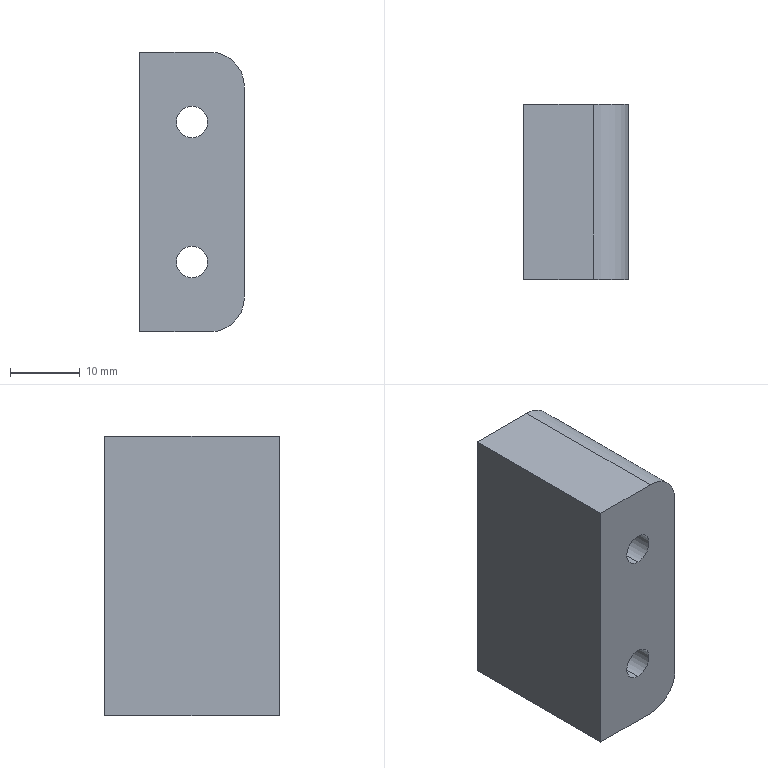Part | SolidWorks | features Extrusion 1, Fillet 1, HoleWzd 1 | 1 solid | 22 faces | box 15 x 25 x 40 mm | volume 13620 mm3 | cylinder 10 | plane 8 | cone 4 | commonest cylinder face diameters 4.5 x4 8 x4 10 x2
STEP:
#1=CARTESIAN_POINT('',(0.,24.975,-14.));
#2=VERTEX_POINT('',#1);
#3=CARTESIAN_POINT('',(0.,24.975,-6.));
#4=VERTEX_POINT('',#3);
#5=CARTESIAN_POINT('',(0.,24.975,-10.));
#6=DIRECTION('',(0.,1.,0.));
#7=DIRECTION('',(0.,0.,1.));
#8=AXIS2_PLACEMENT_3D('',#5,#6,#7);
#9=CIRCLE('',#8,4.);
#10=EDGE_CURVE('',#2,#4,#9,.T.);
#11=ORIENTED_EDGE('',*,*,#10,.F.);
#12=CARTESIAN_POINT('',(0.,25.,-14.025));
#13=VERTEX_POINT('',#12);
#14=CARTESIAN_POINT('',(0.,25.,-14.025));
#15=DIRECTION('',(0.,0.7071,-0.7071));
#16=VECTOR('',#15,1000.);
#17=LINE('',#14,#16);
#18=EDGE_CURVE('',#2,#13,#17,.T.);
#19=ORIENTED_EDGE('',*,*,#18,.T.);
#20=CARTESIAN_POINT('',(0.,25.,-5.975));
#21=VERTEX_POINT('',#20);
#22=CARTESIAN_POINT('',(0.,25.,-10.));
#23=DIRECTION('',(0.,1.,0.));
#24=DIRECTION('',(0.,0.,1.));
#25=AXIS2_PLACEMENT_3D('',#22,#23,#24);
#26=CIRCLE('',#25,4.025);
#27=EDGE_CURVE('',#13,#21,#26,.T.);
#28=ORIENTED_EDGE('',*,*,#27,.T.);
#29=CARTESIAN_POINT('',(0.,25.,-5.975));
#30=DIRECTION('',(0.,0.7071,0.7071));
#31=VECTOR('',#30,1000.);
#32=LINE('',#29,#31);
#33=EDGE_CURVE('',#4,#21,#32,.T.);
#34=ORIENTED_EDGE('',*,*,#33,.F.);
#35=EDGE_LOOP('',(#11,#19,#28,#34));
#36=FACE_OUTER_BOUND('',#35,.T.);
#37=CARTESIAN_POINT('',(0.,25.,-10.));
#38=DIRECTION('',(0.,1.,0.));
#39=DIRECTION('',(0.,0.,1.));
#40=AXIS2_PLACEMENT_3D('',#37,#38,#39);
#41=CONICAL_SURFACE('',#40,4.025,0.7854);
#42=ADVANCED_FACE('',(#36),#41,.F.);
#43=CARTESIAN_POINT('',(0.,20.4,-14.));
#44=VERTEX_POINT('',#43);
#45=CARTESIAN_POINT('',(0.,20.4,-6.));
#46=VERTEX_POINT('',#45);
#47=CARTESIAN_POINT('',(0.,20.4,-10.));
#48=DIRECTION('',(0.,1.,0.));
#49=DIRECTION('',(0.,0.,1.));
#50=AXIS2_PLACEMENT_3D('',#47,#48,#49);
#51=CIRCLE('',#50,4.);
#52=EDGE_CURVE('',#44,#46,#51,.T.);
#53=ORIENTED_EDGE('',*,*,#52,.F.);
#54=CARTESIAN_POINT('',(0.,25.,-14.));
#55=DIRECTION('',(0.,1.,0.));
#56=VECTOR('',#55,1000.);
#57=LINE('',#54,#56);
#58=EDGE_CURVE('',#44,#2,#57,.T.);
#59=ORIENTED_EDGE('',*,*,#58,.T.);
#60=ORIENTED_EDGE('',*,*,#10,.T.);
#61=CARTESIAN_POINT('',(0.,25.,-6.));
#62=DIRECTION('',(0.,1.,0.));
#63=VECTOR('',#62,1000.);
#64=LINE('',#61,#63);
#65=EDGE_CURVE('',#46,#4,#64,.T.);
#66=ORIENTED_EDGE('',*,*,#65,.F.);
#67=EDGE_LOOP('',(#53,#59,#60,#66));
#68=FACE_OUTER_BOUND('',#67,.T.);
#69=CARTESIAN_POINT('',(0.,25.,-10.));
#70=DIRECTION('',(0.,1.,0.));
#71=DIRECTION('',(0.,0.,1.));
#72=AXIS2_PLACEMENT_3D('',#69,#70,#71);
#73=CYLINDRICAL_SURFACE('',#72,4.);
#74=ADVANCED_FACE('',(#68),#73,.F.);
#75=CARTESIAN_POINT('',(0.,0.,-12.25));
#76=VERTEX_POINT('',#75);
#77=CARTESIAN_POINT('',(0.,0.,-7.75));
#78=VERTEX_POINT('',#77);
#79=CARTESIAN_POINT('',(0.,0.,-10.));
#80=DIRECTION('',(0.,1.,0.));
#81=DIRECTION('',(0.,0.,1.));
#82=AXIS2_PLACEMENT_3D('',#79,#80,#81);
#83=CIRCLE('',#82,2.25);
#84=EDGE_CURVE('',#76,#78,#83,.T.);
#85=ORIENTED_EDGE('',*,*,#84,.F.);
#86=CARTESIAN_POINT('',(0.,20.4,-12.25));
#87=VERTEX_POINT('',#86);
#88=CARTESIAN_POINT('',(0.,25.,-12.25));
#89=DIRECTION('',(0.,1.,0.));
#90=VECTOR('',#89,1000.);
#91=LINE('',#88,#90);
#92=EDGE_CURVE('',#76,#87,#91,.T.);
#93=ORIENTED_EDGE('',*,*,#92,.T.);
#94=CARTESIAN_POINT('',(0.,20.4,-7.75));
#95=VERTEX_POINT('',#94);
#96=CARTESIAN_POINT('',(0.,20.4,-10.));
#97=DIRECTION('',(0.,1.,0.));
#98=DIRECTION('',(0.,0.,1.));
#99=AXIS2_PLACEMENT_3D('',#96,#97,#98);
#100=CIRCLE('',#99,2.25);
#101=EDGE_CURVE('',#87,#95,#100,.T.);
#102=ORIENTED_EDGE('',*,*,#101,.T.);
#103=CARTESIAN_POINT('',(0.,25.,-7.75));
#104=DIRECTION('',(0.,1.,0.));
#105=VECTOR('',#104,1000.);
#106=LINE('',#103,#105);
#107=EDGE_CURVE('',#78,#95,#106,.T.);
#108=ORIENTED_EDGE('',*,*,#107,.F.);
#109=EDGE_LOOP('',(#85,#93,#102,#108));
#110=FACE_OUTER_BOUND('',#109,.T.);
#111=CARTESIAN_POINT('',(0.,25.,-10.));
#112=DIRECTION('',(0.,1.,0.));
#113=DIRECTION('',(0.,0.,1.));
#114=AXIS2_PLACEMENT_3D('',#111,#112,#113);
#115=CYLINDRICAL_SURFACE('',#114,2.25);
#116=ADVANCED_FACE('',(#110),#115,.F.);
#117=CARTESIAN_POINT('',(0.,24.975,6.));
#118=VERTEX_POINT('',#117);
#119=CARTESIAN_POINT('',(0.,24.975,14.));
#120=VERTEX_POINT('',#119);
#121=CARTESIAN_POINT('',(0.,24.975,10.));
#122=DIRECTION('',(0.,1.,0.));
#123=DIRECTION('',(0.,0.,1.));
#124=AXIS2_PLACEMENT_3D('',#121,#122,#123);
#125=CIRCLE('',#124,4.);
#126=EDGE_CURVE('',#118,#120,#125,.T.);
#127=ORIENTED_EDGE('',*,*,#126,.F.);
#128=CARTESIAN_POINT('',(0.,25.,5.975));
#129=VERTEX_POINT('',#128);
#130=CARTESIAN_POINT('',(0.,25.,5.975));
#131=DIRECTION('',(0.,0.7071,-0.7071));
#132=VECTOR('',#131,1000.);
#133=LINE('',#130,#132);
#134=EDGE_CURVE('',#118,#129,#133,.T.);
#135=ORIENTED_EDGE('',*,*,#134,.T.);
#136=CARTESIAN_POINT('',(0.,25.,14.025));
#137=VERTEX_POINT('',#136);
#138=CARTESIAN_POINT('',(0.,25.,10.));
#139=DIRECTION('',(0.,1.,0.));
#140=DIRECTION('',(0.,0.,1.));
#141=AXIS2_PLACEMENT_3D('',#138,#139,#140);
#142=CIRCLE('',#141,4.025);
#143=EDGE_CURVE('',#129,#137,#142,.T.);
#144=ORIENTED_EDGE('',*,*,#143,.T.);
#145=CARTESIAN_POINT('',(0.,25.,14.025));
#146=DIRECTION('',(0.,0.7071,0.7071));
#147=VECTOR('',#146,1000.);
#148=LINE('',#145,#147);
#149=EDGE_CURVE('',#120,#137,#148,.T.);
#150=ORIENTED_EDGE('',*,*,#149,.F.);
#151=EDGE_LOOP('',(#127,#135,#144,#150));
#152=FACE_OUTER_BOUND('',#151,.T.);
#153=CARTESIAN_POINT('',(0.,25.,10.));
#154=DIRECTION('',(0.,1.,0.));
#155=DIRECTION('',(0.,0.,1.));
#156=AXIS2_PLACEMENT_3D('',#153,#154,#155);
#157=CONICAL_SURFACE('',#156,4.025,0.7854);
#158=ADVANCED_FACE('',(#152),#157,.F.);
#159=CARTESIAN_POINT('',(0.,20.4,6.));
#160=VERTEX_POINT('',#159);
#161=CARTESIAN_POINT('',(0.,20.4,14.));
#162=VERTEX_POINT('',#161);
#163=CARTESIAN_POINT('',(0.,20.4,10.));
#164=DIRECTION('',(0.,1.,0.));
#165=DIRECTION('',(0.,0.,1.));
#166=AXIS2_PLACEMENT_3D('',#163,#164,#165);
#167=CIRCLE('',#166,4.);
#168=EDGE_CURVE('',#160,#162,#167,.T.);
#169=ORIENTED_EDGE('',*,*,#168,.F.);
#170=CARTESIAN_POINT('',(0.,25.,6.));
#171=DIRECTION('',(0.,1.,0.));
#172=VECTOR('',#171,1000.);
#173=LINE('',#170,#172);
#174=EDGE_CURVE('',#160,#118,#173,.T.);
#175=ORIENTED_EDGE('',*,*,#174,.T.);
#176=ORIENTED_EDGE('',*,*,#126,.T.);
#177=CARTESIAN_POINT('',(0.,25.,14.));
#178=DIRECTION('',(0.,1.,0.));
#179=VECTOR('',#178,1000.);
#180=LINE('',#177,#179);
#181=EDGE_CURVE('',#162,#120,#180,.T.);
#182=ORIENTED_EDGE('',*,*,#181,.F.);
#183=EDGE_LOOP('',(#169,#175,#176,#182));
#184=FACE_OUTER_BOUND('',#183,.T.);
#185=CARTESIAN_POINT('',(0.,25.,10.));
#186=DIRECTION('',(0.,1.,0.));
#187=DIRECTION('',(0.,0.,1.));
#188=AXIS2_PLACEMENT_3D('',#185,#186,#187);
#189=CYLINDRICAL_SURFACE('',#188,4.);
#190=ADVANCED_FACE('',(#184),#189,.F.);
#191=CARTESIAN_POINT('',(0.,0.,7.75));
#192=VERTEX_POINT('',#191);
#193=CARTESIAN_POINT('',(0.,0.,12.25));
#194=VERTEX_POINT('',#193);
#195=CARTESIAN_POINT('',(0.,0.,10.));
#196=DIRECTION('',(0.,1.,0.));
#197=DIRECTION('',(0.,0.,1.));
#198=AXIS2_PLACEMENT_3D('',#195,#196,#197);
#199=CIRCLE('',#198,2.25);
#200=EDGE_CURVE('',#192,#194,#199,.T.);
#201=ORIENTED_EDGE('',*,*,#200,.F.);
#202=CARTESIAN_POINT('',(0.,20.4,7.75));
#203=VERTEX_POINT('',#202);
#204=CARTESIAN_POINT('',(0.,25.,7.75));
#205=DIRECTION('',(0.,1.,0.));
#206=VECTOR('',#205,1000.);
#207=LINE('',#204,#206);
#208=EDGE_CURVE('',#192,#203,#207,.T.);
#209=ORIENTED_EDGE('',*,*,#208,.T.);
#210=CARTESIAN_POINT('',(0.,20.4,12.25));
#211=VERTEX_POINT('',#210);
#212=CARTESIAN_POINT('',(0.,20.4,10.));
#213=DIRECTION('',(0.,1.,0.));
#214=DIRECTION('',(0.,0.,1.));
#215=AXIS2_PLACEMENT_3D('',#212,#213,#214);
#216=CIRCLE('',#215,2.25);
#217=EDGE_CURVE('',#203,#211,#216,.T.);
#218=ORIENTED_EDGE('',*,*,#217,.T.);
#219=CARTESIAN_POINT('',(0.,25.,12.25));
#220=DIRECTION('',(0.,1.,0.));
#221=VECTOR('',#220,1000.);
#222=LINE('',#219,#221);
#223=EDGE_CURVE('',#194,#211,#222,.T.);
#224=ORIENTED_EDGE('',*,*,#223,.F.);
#225=EDGE_LOOP('',(#201,#209,#218,#224));
#226=FACE_OUTER_BOUND('',#225,.T.);
#227=CARTESIAN_POINT('',(0.,25.,10.));
#228=DIRECTION('',(0.,1.,0.));
#229=DIRECTION('',(0.,0.,1.));
#230=AXIS2_PLACEMENT_3D('',#227,#228,#229);
#231=CYLINDRICAL_SURFACE('',#230,2.25);
#232=ADVANCED_FACE('',(#226),#231,.F.);
#233=CARTESIAN_POINT('',(7.5,25.,15.));
#234=VERTEX_POINT('',#233);
#235=CARTESIAN_POINT('',(7.5,25.,-15.));
#236=VERTEX_POINT('',#235);
#237=CARTESIAN_POINT('',(7.5,25.,20.));
#238=DIRECTION('',(0.,0.,-1.));
#239=VECTOR('',#238,1000.);
#240=LINE('',#237,#239);
#241=EDGE_CURVE('',#234,#236,#240,.T.);
#242=ORIENTED_EDGE('',*,*,#241,.F.);
#243=CARTESIAN_POINT('',(7.5,0.,15.));
#244=VERTEX_POINT('',#243);
#245=CARTESIAN_POINT('',(7.5,25.,15.));
#246=DIRECTION('',(0.,-1.,0.));
#247=VECTOR('',#246,1000.);
#248=LINE('',#245,#247);
#249=EDGE_CURVE('',#234,#244,#248,.T.);
#250=ORIENTED_EDGE('',*,*,#249,.T.);
#251=CARTESIAN_POINT('',(7.5,0.,-15.));
#252=VERTEX_POINT('',#251);
#253=CARTESIAN_POINT('',(7.5,0.,20.));
#254=DIRECTION('',(0.,0.,-1.));
#255=VECTOR('',#254,1000.);
#256=LINE('',#253,#255);
#257=EDGE_CURVE('',#244,#252,#256,.T.);
#258=ORIENTED_EDGE('',*,*,#257,.T.);
#259=CARTESIAN_POINT('',(7.5,25.,-15.));
#260=DIRECTION('',(0.,1.,0.));
#261=VECTOR('',#260,1000.);
#262=LINE('',#259,#261);
#263=EDGE_CURVE('',#252,#236,#262,.T.);
#264=ORIENTED_EDGE('',*,*,#263,.T.);
#265=EDGE_LOOP('',(#242,#250,#258,#264));
#266=FACE_OUTER_BOUND('',#265,.T.);
#267=CARTESIAN_POINT('',(7.5,25.,20.));
#268=DIRECTION('',(-1.,0.,0.));
#269=DIRECTION('',(0.,0.,1.));
#270=AXIS2_PLACEMENT_3D('',#267,#268,#269);
#271=PLANE('',#270);
#272=ADVANCED_FACE('',(#266),#271,.F.);
#273=CARTESIAN_POINT('',(2.5,25.,-20.));
#274=VERTEX_POINT('',#273);
#275=CARTESIAN_POINT('',(-7.5,25.,-20.));
#276=VERTEX_POINT('',#275);
#277=CARTESIAN_POINT('',(-7.5,25.,-20.));
#278=DIRECTION('',(-1.,0.,0.));
#279=VECTOR('',#278,1000.);
#280=LINE('',#277,#279);
#281=EDGE_CURVE('',#274,#276,#280,.T.);
#282=ORIENTED_EDGE('',*,*,#281,.F.);
#283=CARTESIAN_POINT('',(2.5,0.,-20.));
#284=VERTEX_POINT('',#283);
#285=CARTESIAN_POINT('',(2.5,25.,-20.));
#286=DIRECTION('',(0.,-1.,0.));
#287=VECTOR('',#286,1000.);
#288=LINE('',#285,#287);
#289=EDGE_CURVE('',#274,#284,#288,.T.);
#290=ORIENTED_EDGE('',*,*,#289,.T.);
#291=CARTESIAN_POINT('',(-7.5,0.,-20.));
#292=VERTEX_POINT('',#291);
#293=CARTESIAN_POINT('',(-7.5,0.,-20.));
#294=DIRECTION('',(-1.,0.,0.));
#295=VECTOR('',#294,1000.);
#296=LINE('',#293,#295);
#297=EDGE_CURVE('',#284,#292,#296,.T.);
#298=ORIENTED_EDGE('',*,*,#297,.T.);
#299=CARTESIAN_POINT('',(-7.5,25.,-20.));
#300=DIRECTION('',(0.,-1.,0.));
#301=VECTOR('',#300,1000.);
#302=LINE('',#299,#301);
#303=EDGE_CURVE('',#276,#292,#302,.T.);
#304=ORIENTED_EDGE('',*,*,#303,.F.);
#305=EDGE_LOOP('',(#282,#290,#298,#304));
#306=FACE_OUTER_BOUND('',#305,.T.);
#307=CARTESIAN_POINT('',(-7.5,25.,-20.));
#308=DIRECTION('',(0.,0.,1.));
#309=DIRECTION('',(1.,0.,0.));
#310=AXIS2_PLACEMENT_3D('',#307,#308,#309);
#311=PLANE('',#310);
#312=ADVANCED_FACE('',(#306),#311,.F.);
#313=CARTESIAN_POINT('',(-7.5,0.,20.));
#314=VERTEX_POINT('',#313);
#315=CARTESIAN_POINT('',(-7.5,0.,20.));
#316=DIRECTION('',(0.,0.,1.));
#317=VECTOR('',#316,1000.);
#318=LINE('',#315,#317);
#319=EDGE_CURVE('',#292,#314,#318,.T.);
#320=ORIENTED_EDGE('',*,*,#319,.T.);
#321=CARTESIAN_POINT('',(-7.5,25.,20.));
#322=VERTEX_POINT('',#321);
#323=CARTESIAN_POINT('',(-7.5,25.,20.));
#324=DIRECTION('',(0.,-1.,0.));
#325=VECTOR('',#324,1000.);
#326=LINE('',#323,#325);
#327=EDGE_CURVE('',#322,#314,#326,.T.);
#328=ORIENTED_EDGE('',*,*,#327,.F.);
#329=CARTESIAN_POINT('',(-7.5,25.,20.));
#330=DIRECTION('',(0.,0.,1.));
#331=VECTOR('',#330,1000.);
#332=LINE('',#329,#331);
#333=EDGE_CURVE('',#276,#322,#332,.T.);
#334=ORIENTED_EDGE('',*,*,#333,.F.);
#335=ORIENTED_EDGE('',*,*,#303,.T.);
#336=EDGE_LOOP('',(#320,#328,#334,#335));
#337=FACE_OUTER_BOUND('',#336,.T.);
#338=CARTESIAN_POINT('',(-7.5,25.,20.));
#339=DIRECTION('',(1.,0.,0.));
#340=DIRECTION('',(0.,0.,-1.));
#341=AXIS2_PLACEMENT_3D('',#338,#339,#340);
#342=PLANE('',#341);
#343=ADVANCED_FACE('',(#337),#342,.F.);
#344=CARTESIAN_POINT('',(2.5,0.,20.));
#345=VERTEX_POINT('',#344);
#346=CARTESIAN_POINT('',(-7.5,0.,20.));
#347=DIRECTION('',(1.,0.,0.));
#348=VECTOR('',#347,1000.);
#349=LINE('',#346,#348);
#350=EDGE_CURVE('',#314,#345,#349,.T.);
#351=ORIENTED_EDGE('',*,*,#350,.T.);
#352=CARTESIAN_POINT('',(2.5,25.,20.));
#353=VERTEX_POINT('',#352);
#354=CARTESIAN_POINT('',(2.5,25.,20.));
#355=DIRECTION('',(0.,1.,0.));
#356=VECTOR('',#355,1000.);
#357=LINE('',#354,#356);
#358=EDGE_CURVE('',#345,#353,#357,.T.);
#359=ORIENTED_EDGE('',*,*,#358,.T.);
#360=CARTESIAN_POINT('',(-7.5,25.,20.));
#361=DIRECTION('',(1.,0.,0.));
#362=VECTOR('',#361,1000.);
#363=LINE('',#360,#362);
#364=EDGE_CURVE('',#322,#353,#363,.T.);
#365=ORIENTED_EDGE('',*,*,#364,.F.);
#366=ORIENTED_EDGE('',*,*,#327,.T.);
#367=EDGE_LOOP('',(#351,#359,#365,#366));
#368=FACE_OUTER_BOUND('',#367,.T.);
#369=CARTESIAN_POINT('',(-7.5,25.,20.));
#370=DIRECTION('',(0.,0.,-1.));
#371=DIRECTION('',(-1.,0.,0.));
#372=AXIS2_PLACEMENT_3D('',#369,#370,#371);
#373=PLANE('',#372);
#374=ADVANCED_FACE('',(#368),#373,.F.);
#375=CARTESIAN_POINT('',(0.,25.,-10.));
#376=DIRECTION('',(0.,1.,0.));
#377=DIRECTION('',(0.,0.,1.));
#378=AXIS2_PLACEMENT_3D('',#375,#376,#377);
#379=CIRCLE('',#378,4.025);
#380=EDGE_CURVE('',#21,#13,#379,.T.);
#381=ORIENTED_EDGE('',*,*,#380,.F.);
#382=ORIENTED_EDGE('',*,*,#27,.F.);
#383=EDGE_LOOP('',(#381,#382));
#384=FACE_BOUND('',#383,.T.);
#385=CARTESIAN_POINT('',(0.,25.,10.));
#386=DIRECTION('',(0.,1.,0.));
#387=DIRECTION('',(0.,0.,1.));
#388=AXIS2_PLACEMENT_3D('',#385,#386,#387);
#389=CIRCLE('',#388,4.025);
#390=EDGE_CURVE('',#137,#129,#389,.T.);
#391=ORIENTED_EDGE('',*,*,#390,.F.);
#392=ORIENTED_EDGE('',*,*,#143,.F.);
#393=EDGE_LOOP('',(#391,#392));
#394=FACE_BOUND('',#393,.T.);
#395=ORIENTED_EDGE('',*,*,#364,.T.);
#396=CARTESIAN_POINT('',(2.5,25.,15.));
#397=DIRECTION('',(0.,1.,0.));
#398=DIRECTION('',(0.,0.,-1.));
#399=AXIS2_PLACEMENT_3D('',#396,#397,#398);
#400=CIRCLE('',#399,5.);
#401=EDGE_CURVE('',#353,#234,#400,.T.);
#402=ORIENTED_EDGE('',*,*,#401,.T.);
#403=ORIENTED_EDGE('',*,*,#241,.T.);
#404=CARTESIAN_POINT('',(2.5,25.,-15.));
#405=DIRECTION('',(0.,1.,0.));
#406=DIRECTION('',(0.,0.,-1.));
#407=AXIS2_PLACEMENT_3D('',#404,#405,#406);
#408=CIRCLE('',#407,5.);
#409=EDGE_CURVE('',#236,#274,#408,.T.);
#410=ORIENTED_EDGE('',*,*,#409,.T.);
#411=ORIENTED_EDGE('',*,*,#281,.T.);
#412=ORIENTED_EDGE('',*,*,#333,.T.);
#413=EDGE_LOOP('',(#395,#402,#403,#410,#411,#412));
#414=FACE_OUTER_BOUND('',#413,.T.);
#415=CARTESIAN_POINT('',(0.,25.,0.));
#416=DIRECTION('',(0.,-1.,0.));
#417=DIRECTION('',(0.,0.,-1.));
#418=AXIS2_PLACEMENT_3D('',#415,#416,#417);
#419=PLANE('',#418);
#420=ADVANCED_FACE('',(#384,#394,#414),#419,.F.);
#421=CARTESIAN_POINT('',(0.,0.,-10.));
#422=DIRECTION('',(0.,1.,0.));
#423=DIRECTION('',(0.,0.,1.));
#424=AXIS2_PLACEMENT_3D('',#421,#422,#423);
#425=CIRCLE('',#424,2.25);
#426=EDGE_CURVE('',#78,#76,#425,.T.);
#427=ORIENTED_EDGE('',*,*,#426,.T.);
#428=ORIENTED_EDGE('',*,*,#84,.T.);
#429=EDGE_LOOP('',(#427,#428));
#430=FACE_BOUND('',#429,.T.);
#431=CARTESIAN_POINT('',(0.,0.,10.));
#432=DIRECTION('',(0.,1.,0.));
#433=DIRECTION('',(0.,0.,1.));
#434=AXIS2_PLACEMENT_3D('',#431,#432,#433);
#435=CIRCLE('',#434,2.25);
#436=EDGE_CURVE('',#194,#192,#435,.T.);
#437=ORIENTED_EDGE('',*,*,#436,.T.);
#438=ORIENTED_EDGE('',*,*,#200,.T.);
#439=EDGE_LOOP('',(#437,#438));
#440=FACE_BOUND('',#439,.T.);
#441=ORIENTED_EDGE('',*,*,#257,.F.);
#442=CARTESIAN_POINT('',(2.5,0.,15.));
#443=DIRECTION('',(0.,-1.,0.));
#444=DIRECTION('',(0.,0.,-1.));
#445=AXIS2_PLACEMENT_3D('',#442,#443,#444);
#446=CIRCLE('',#445,5.);
#447=EDGE_CURVE('',#244,#345,#446,.T.);
#448=ORIENTED_EDGE('',*,*,#447,.T.);
#449=ORIENTED_EDGE('',*,*,#350,.F.);
#450=ORIENTED_EDGE('',*,*,#319,.F.);
#451=ORIENTED_EDGE('',*,*,#297,.F.);
#452=CARTESIAN_POINT('',(2.5,0.,-15.));
#453=DIRECTION('',(0.,-1.,0.));
#454=DIRECTION('',(0.,0.,-1.));
#455=AXIS2_PLACEMENT_3D('',#452,#453,#454);
#456=CIRCLE('',#455,5.);
#457=EDGE_CURVE('',#284,#252,#456,.T.);
#458=ORIENTED_EDGE('',*,*,#457,.T.);
#459=EDGE_LOOP('',(#441,#448,#449,#450,#451,#458));
#460=FACE_OUTER_BOUND('',#459,.T.);
#461=CARTESIAN_POINT('',(0.,0.,0.));
#462=DIRECTION('',(0.,-1.,0.));
#463=DIRECTION('',(0.,0.,-1.));
#464=AXIS2_PLACEMENT_3D('',#461,#462,#463);
#465=PLANE('',#464);
#466=ADVANCED_FACE('',(#430,#440,#460),#465,.T.);
#467=ORIENTED_EDGE('',*,*,#401,.F.);
#468=ORIENTED_EDGE('',*,*,#358,.F.);
#469=ORIENTED_EDGE('',*,*,#447,.F.);
#470=ORIENTED_EDGE('',*,*,#249,.F.);
#471=EDGE_LOOP('',(#467,#468,#469,#470));
#472=FACE_OUTER_BOUND('',#471,.T.);
#473=CARTESIAN_POINT('',(2.5,25.,15.));
#474=DIRECTION('',(0.,-1.,0.));
#475=DIRECTION('',(0.,0.,-1.));
#476=AXIS2_PLACEMENT_3D('',#473,#474,#475);
#477=CYLINDRICAL_SURFACE('',#476,5.);
#478=ADVANCED_FACE('',(#472),#477,.T.);
#479=ORIENTED_EDGE('',*,*,#409,.F.);
#480=ORIENTED_EDGE('',*,*,#263,.F.);
#481=ORIENTED_EDGE('',*,*,#457,.F.);
#482=ORIENTED_EDGE('',*,*,#289,.F.);
#483=EDGE_LOOP('',(#479,#480,#481,#482));
#484=FACE_OUTER_BOUND('',#483,.T.);
#485=CARTESIAN_POINT('',(2.5,25.,-15.));
#486=DIRECTION('',(0.,-1.,0.));
#487=DIRECTION('',(0.,0.,-1.));
#488=AXIS2_PLACEMENT_3D('',#485,#486,#487);
#489=CYLINDRICAL_SURFACE('',#488,5.);
#490=ADVANCED_FACE('',(#484),#489,.T.);
#491=ORIENTED_EDGE('',*,*,#208,.F.);
#492=ORIENTED_EDGE('',*,*,#436,.F.);
#493=ORIENTED_EDGE('',*,*,#223,.T.);
#494=CARTESIAN_POINT('',(0.,20.4,10.));
#495=DIRECTION('',(0.,1.,0.));
#496=DIRECTION('',(0.,0.,1.));
#497=AXIS2_PLACEMENT_3D('',#494,#495,#496);
#498=CIRCLE('',#497,2.25);
#499=EDGE_CURVE('',#211,#203,#498,.T.);
#500=ORIENTED_EDGE('',*,*,#499,.T.);
#501=EDGE_LOOP('',(#491,#492,#493,#500));
#502=FACE_OUTER_BOUND('',#501,.T.);
#503=CARTESIAN_POINT('',(0.,25.,10.));
#504=DIRECTION('',(0.,1.,0.));
#505=DIRECTION('',(0.,0.,1.));
#506=AXIS2_PLACEMENT_3D('',#503,#504,#505);
#507=CYLINDRICAL_SURFACE('',#506,2.25);
#508=ADVANCED_FACE('',(#502),#507,.F.);
#509=ORIENTED_EDGE('',*,*,#499,.F.);
#510=ORIENTED_EDGE('',*,*,#217,.F.);
#511=EDGE_LOOP('',(#509,#510));
#512=FACE_BOUND('',#511,.T.);
#513=CARTESIAN_POINT('',(0.,20.4,10.));
#514=DIRECTION('',(0.,1.,0.));
#515=DIRECTION('',(0.,0.,1.));
#516=AXIS2_PLACEMENT_3D('',#513,#514,#515);
#517=CIRCLE('',#516,4.);
#518=EDGE_CURVE('',#162,#160,#517,.T.);
#519=ORIENTED_EDGE('',*,*,#518,.T.);
#520=ORIENTED_EDGE('',*,*,#168,.T.);
#521=EDGE_LOOP('',(#519,#520));
#522=FACE_OUTER_BOUND('',#521,.T.);
#523=CARTESIAN_POINT('',(4.,20.4,10.));
#524=DIRECTION('',(0.,-1.,0.));
#525=DIRECTION('',(0.,0.,-1.));
#526=AXIS2_PLACEMENT_3D('',#523,#524,#525);
#527=PLANE('',#526);
#528=ADVANCED_FACE('',(#512,#522),#527,.F.);
#529=ORIENTED_EDGE('',*,*,#174,.F.);
#530=ORIENTED_EDGE('',*,*,#518,.F.);
#531=ORIENTED_EDGE('',*,*,#181,.T.);
#532=CARTESIAN_POINT('',(0.,24.975,10.));
#533=DIRECTION('',(0.,1.,0.));
#534=DIRECTION('',(0.,0.,1.));
#535=AXIS2_PLACEMENT_3D('',#532,#533,#534);
#536=CIRCLE('',#535,4.);
#537=EDGE_CURVE('',#120,#118,#536,.T.);
#538=ORIENTED_EDGE('',*,*,#537,.T.);
#539=EDGE_LOOP('',(#529,#530,#531,#538));
#540=FACE_OUTER_BOUND('',#539,.T.);
#541=CARTESIAN_POINT('',(0.,25.,10.));
#542=DIRECTION('',(0.,1.,0.));
#543=DIRECTION('',(0.,0.,1.));
#544=AXIS2_PLACEMENT_3D('',#541,#542,#543);
#545=CYLINDRICAL_SURFACE('',#544,4.);
#546=ADVANCED_FACE('',(#540),#545,.F.);
#547=ORIENTED_EDGE('',*,*,#134,.F.);
#548=ORIENTED_EDGE('',*,*,#537,.F.);
#549=ORIENTED_EDGE('',*,*,#149,.T.);
#550=ORIENTED_EDGE('',*,*,#390,.T.);
#551=EDGE_LOOP('',(#547,#548,#549,#550));
#552=FACE_OUTER_BOUND('',#551,.T.);
#553=CARTESIAN_POINT('',(0.,25.,10.));
#554=DIRECTION('',(0.,1.,0.));
#555=DIRECTION('',(0.,0.,1.));
#556=AXIS2_PLACEMENT_3D('',#553,#554,#555);
#557=CONICAL_SURFACE('',#556,4.025,0.7854);
#558=ADVANCED_FACE('',(#552),#557,.F.);
#559=ORIENTED_EDGE('',*,*,#92,.F.);
#560=ORIENTED_EDGE('',*,*,#426,.F.);
#561=ORIENTED_EDGE('',*,*,#107,.T.);
#562=CARTESIAN_POINT('',(0.,20.4,-10.));
#563=DIRECTION('',(0.,1.,0.));
#564=DIRECTION('',(0.,0.,1.));
#565=AXIS2_PLACEMENT_3D('',#562,#563,#564);
#566=CIRCLE('',#565,2.25);
#567=EDGE_CURVE('',#95,#87,#566,.T.);
#568=ORIENTED_EDGE('',*,*,#567,.T.);
#569=EDGE_LOOP('',(#559,#560,#561,#568));
#570=FACE_OUTER_BOUND('',#569,.T.);
#571=CARTESIAN_POINT('',(0.,25.,-10.));
#572=DIRECTION('',(0.,1.,0.));
#573=DIRECTION('',(0.,0.,1.));
#574=AXIS2_PLACEMENT_3D('',#571,#572,#573);
#575=CYLINDRICAL_SURFACE('',#574,2.25);
#576=ADVANCED_FACE('',(#570),#575,.F.);
#577=ORIENTED_EDGE('',*,*,#567,.F.);
#578=ORIENTED_EDGE('',*,*,#101,.F.);
#579=EDGE_LOOP('',(#577,#578));
#580=FACE_BOUND('',#579,.T.);
#581=CARTESIAN_POINT('',(0.,20.4,-10.));
#582=DIRECTION('',(0.,1.,0.));
#583=DIRECTION('',(0.,0.,1.));
#584=AXIS2_PLACEMENT_3D('',#581,#582,#583);
#585=CIRCLE('',#584,4.);
#586=EDGE_CURVE('',#46,#44,#585,.T.);
#587=ORIENTED_EDGE('',*,*,#586,.T.);
#588=ORIENTED_EDGE('',*,*,#52,.T.);
#589=EDGE_LOOP('',(#587,#588));
#590=FACE_OUTER_BOUND('',#589,.T.);
#591=CARTESIAN_POINT('',(4.,20.4,-10.));
#592=DIRECTION('',(0.,-1.,0.));
#593=DIRECTION('',(0.,0.,-1.));
#594=AXIS2_PLACEMENT_3D('',#591,#592,#593);
#595=PLANE('',#594);
#596=ADVANCED_FACE('',(#580,#590),#595,.F.);
#597=ORIENTED_EDGE('',*,*,#58,.F.);
#598=ORIENTED_EDGE('',*,*,#586,.F.);
#599=ORIENTED_EDGE('',*,*,#65,.T.);
#600=CARTESIAN_POINT('',(0.,24.975,-10.));
#601=DIRECTION('',(0.,1.,0.));
#602=DIRECTION('',(0.,0.,1.));
#603=AXIS2_PLACEMENT_3D('',#600,#601,#602);
#604=CIRCLE('',#603,4.);
#605=EDGE_CURVE('',#4,#2,#604,.T.);
#606=ORIENTED_EDGE('',*,*,#605,.T.);
#607=EDGE_LOOP('',(#597,#598,#599,#606));
#608=FACE_OUTER_BOUND('',#607,.T.);
#609=CARTESIAN_POINT('',(0.,25.,-10.));
#610=DIRECTION('',(0.,1.,0.));
#611=DIRECTION('',(0.,0.,1.));
#612=AXIS2_PLACEMENT_3D('',#609,#610,#611);
#613=CYLINDRICAL_SURFACE('',#612,4.);
#614=ADVANCED_FACE('',(#608),#613,.F.);
#615=ORIENTED_EDGE('',*,*,#18,.F.);
#616=ORIENTED_EDGE('',*,*,#605,.F.);
#617=ORIENTED_EDGE('',*,*,#33,.T.);
#618=ORIENTED_EDGE('',*,*,#380,.T.);
#619=EDGE_LOOP('',(#615,#616,#617,#618));
#620=FACE_OUTER_BOUND('',#619,.T.);
#621=CARTESIAN_POINT('',(0.,25.,-10.));
#622=DIRECTION('',(0.,1.,0.));
#623=DIRECTION('',(0.,0.,1.));
#624=AXIS2_PLACEMENT_3D('',#621,#622,#623);
#625=CONICAL_SURFACE('',#624,4.025,0.7854);
#626=ADVANCED_FACE('',(#620),#625,.F.);
#627=CLOSED_SHELL('',(#42,#74,#116,#158,#190,#232,#272,#312,#343,#374,#420,#466,#478,#490,#508,#528,#546,#558,#576,#596,#614,#626));
#628=MANIFOLD_SOLID_BREP('',#627);
#629=CARTESIAN_POINT('',(0.,0.,0.));
#630=DIRECTION('',(0.,0.,1.));
#631=DIRECTION('',(1.,0.,0.));
#632=AXIS2_PLACEMENT_3D('',#629,#630,#631);
#633=(LENGTH_UNIT()NAMED_UNIT(*)SI_UNIT(.MILLI.,.METRE.));
#634=UNCERTAINTY_MEASURE_WITH_UNIT(LENGTH_MEASURE(0.00001),#633,'','');
#635=(NAMED_UNIT(*)PLANE_ANGLE_UNIT()SI_UNIT($,.RADIAN.));
#636=(NAMED_UNIT(*)SI_UNIT($,.STERADIAN.)SOLID_ANGLE_UNIT());
#637=(GEOMETRIC_REPRESENTATION_CONTEXT(3)GLOBAL_UNCERTAINTY_ASSIGNED_CONTEXT((#634))GLOBAL_UNIT_ASSIGNED_CONTEXT((#633,#635,#636))REPRESENTATION_CONTEXT('',''));
#638=ADVANCED_BREP_SHAPE_REPRESENTATION('',(#628,#632),#637);